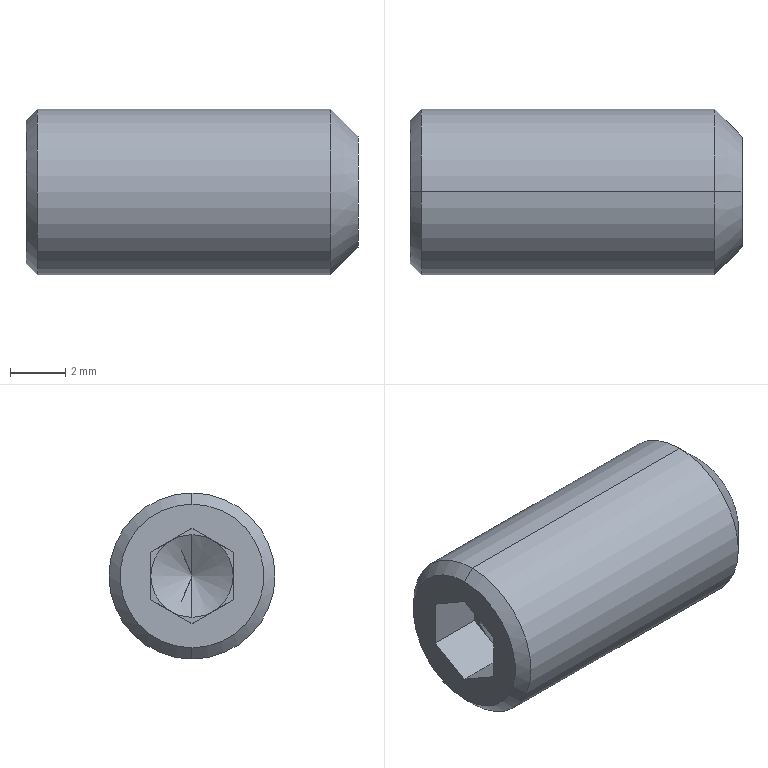Part | SolidWorks | features RevCut 2, Cut 1, LPattern 1, Revolution 1 | 1 solid | 22 faces | box 12 x 6 x 6 mm | volume 312.089 mm3 | plane 14 | cone 6 | cylinder 2 | commonest cylinder face diameters 6 x2
STEP:
#1=CARTESIAN_POINT('',(2.86,0.,0.));
#2=VERTEX_POINT('',#1);
#3=CARTESIAN_POINT('',(2.,0.,1.49));
#4=VERTEX_POINT('',#3);
#5=CARTESIAN_POINT('',(2.86,0.,0.));
#6=DIRECTION('',(-0.5,0.,0.866));
#7=VECTOR('',#6,1000.);
#8=LINE('',#5,#7);
#9=EDGE_CURVE('',#2,#4,#8,.T.);
#10=ORIENTED_EDGE('',*,*,#9,.F.);
#11=CARTESIAN_POINT('',(2.,0.,-1.49));
#12=VERTEX_POINT('',#11);
#13=CARTESIAN_POINT('',(2.86,0.,0.));
#14=DIRECTION('',(-0.5,0.,-0.866));
#15=VECTOR('',#14,1000.);
#16=LINE('',#13,#15);
#17=EDGE_CURVE('',#2,#12,#16,.T.);
#18=ORIENTED_EDGE('',*,*,#17,.T.);
#19=CARTESIAN_POINT('',(2.,-0.7448,-1.29));
#20=VERTEX_POINT('',#19);
#21=CARTESIAN_POINT('',(2.,0.,0.));
#22=DIRECTION('',(-1.,0.,0.));
#23=DIRECTION('',(0.,0.,1.));
#24=AXIS2_PLACEMENT_3D('',#21,#22,#23);
#25=CIRCLE('',#24,1.49);
#26=EDGE_CURVE('',#12,#20,#25,.T.);
#27=ORIENTED_EDGE('',*,*,#26,.T.);
#28=CARTESIAN_POINT('',(2.,-1.49,0.));
#29=VERTEX_POINT('',#28);
#30=CARTESIAN_POINT('',(2.,0.,0.));
#31=DIRECTION('',(-1.,0.,0.));
#32=DIRECTION('',(0.,0.,1.));
#33=AXIS2_PLACEMENT_3D('',#30,#31,#32);
#34=CIRCLE('',#33,1.49);
#35=EDGE_CURVE('',#20,#29,#34,.T.);
#36=ORIENTED_EDGE('',*,*,#35,.T.);
#37=CARTESIAN_POINT('',(2.,-0.7448,1.29));
#38=VERTEX_POINT('',#37);
#39=CARTESIAN_POINT('',(2.,0.,0.));
#40=DIRECTION('',(-1.,0.,0.));
#41=DIRECTION('',(0.,0.,1.));
#42=AXIS2_PLACEMENT_3D('',#39,#40,#41);
#43=CIRCLE('',#42,1.49);
#44=EDGE_CURVE('',#29,#38,#43,.T.);
#45=ORIENTED_EDGE('',*,*,#44,.T.);
#46=CARTESIAN_POINT('',(2.,0.,0.));
#47=DIRECTION('',(-1.,0.,0.));
#48=DIRECTION('',(0.,0.,1.));
#49=AXIS2_PLACEMENT_3D('',#46,#47,#48);
#50=CIRCLE('',#49,1.49);
#51=EDGE_CURVE('',#38,#4,#50,.T.);
#52=ORIENTED_EDGE('',*,*,#51,.T.);
#53=EDGE_LOOP('',(#10,#18,#27,#36,#45,#52));
#54=FACE_OUTER_BOUND('',#53,.T.);
#55=CARTESIAN_POINT('',(-997.14,0.,0.));
#56=DIRECTION('',(-1.,0.,0.));
#57=DIRECTION('',(0.,0.,1.));
#58=AXIS2_PLACEMENT_3D('',#55,#56,#57);
#59=CONICAL_SURFACE('',#58,1732.051,1.047);
#60=ADVANCED_FACE('',(#54),#59,.F.);
#61=CARTESIAN_POINT('',(0.,0.,2.598));
#62=VERTEX_POINT('',#61);
#63=CARTESIAN_POINT('',(0.,0.,-2.598));
#64=VERTEX_POINT('',#63);
#65=CARTESIAN_POINT('',(0.,0.,0.));
#66=DIRECTION('',(-1.,0.,0.));
#67=DIRECTION('',(0.,0.,1.));
#68=AXIS2_PLACEMENT_3D('',#65,#66,#67);
#69=CIRCLE('',#68,2.598);
#70=EDGE_CURVE('',#62,#64,#69,.T.);
#71=ORIENTED_EDGE('',*,*,#70,.F.);
#72=CARTESIAN_POINT('',(0.402,0.,3.));
#73=VERTEX_POINT('',#72);
#74=CARTESIAN_POINT('',(0.402,0.,3.));
#75=DIRECTION('',(0.7071,0.,0.7071));
#76=VECTOR('',#75,1000.);
#77=LINE('',#74,#76);
#78=EDGE_CURVE('',#62,#73,#77,.T.);
#79=ORIENTED_EDGE('',*,*,#78,.T.);
#80=CARTESIAN_POINT('',(0.402,0.,-3.));
#81=VERTEX_POINT('',#80);
#82=CARTESIAN_POINT('',(0.402,0.,0.));
#83=DIRECTION('',(-1.,0.,0.));
#84=DIRECTION('',(0.,0.,1.));
#85=AXIS2_PLACEMENT_3D('',#82,#83,#84);
#86=CIRCLE('',#85,3.);
#87=EDGE_CURVE('',#73,#81,#86,.T.);
#88=ORIENTED_EDGE('',*,*,#87,.T.);
#89=CARTESIAN_POINT('',(0.402,0.,-3.));
#90=DIRECTION('',(0.7071,0.,-0.7071));
#91=VECTOR('',#90,1000.);
#92=LINE('',#89,#91);
#93=EDGE_CURVE('',#64,#81,#92,.T.);
#94=ORIENTED_EDGE('',*,*,#93,.F.);
#95=EDGE_LOOP('',(#71,#79,#88,#94));
#96=FACE_OUTER_BOUND('',#95,.T.);
#97=CARTESIAN_POINT('',(0.402,0.,0.));
#98=DIRECTION('',(1.,0.,0.));
#99=DIRECTION('',(0.,0.,-1.));
#100=AXIS2_PLACEMENT_3D('',#97,#98,#99);
#101=CONICAL_SURFACE('',#100,3.,0.7854);
#102=ADVANCED_FACE('',(#96),#101,.T.);
#103=CARTESIAN_POINT('',(11.,0.,3.));
#104=VERTEX_POINT('',#103);
#105=CARTESIAN_POINT('',(11.,0.,-3.));
#106=VERTEX_POINT('',#105);
#107=CARTESIAN_POINT('',(11.,0.,0.));
#108=DIRECTION('',(-1.,0.,0.));
#109=DIRECTION('',(0.,0.,1.));
#110=AXIS2_PLACEMENT_3D('',#107,#108,#109);
#111=CIRCLE('',#110,3.);
#112=EDGE_CURVE('',#104,#106,#111,.T.);
#113=ORIENTED_EDGE('',*,*,#112,.T.);
#114=CARTESIAN_POINT('',(-0.2778,0.,-3.));
#115=DIRECTION('',(-1.,0.,0.));
#116=VECTOR('',#115,1000.);
#117=LINE('',#114,#116);
#118=EDGE_CURVE('',#106,#81,#117,.T.);
#119=ORIENTED_EDGE('',*,*,#118,.T.);
#120=ORIENTED_EDGE('',*,*,#87,.F.);
#121=CARTESIAN_POINT('',(-0.2778,0.,3.));
#122=DIRECTION('',(-1.,0.,0.));
#123=VECTOR('',#122,1000.);
#124=LINE('',#121,#123);
#125=EDGE_CURVE('',#104,#73,#124,.T.);
#126=ORIENTED_EDGE('',*,*,#125,.F.);
#127=EDGE_LOOP('',(#113,#119,#120,#126));
#128=FACE_OUTER_BOUND('',#127,.T.);
#129=CARTESIAN_POINT('',(-0.2778,0.,0.));
#130=DIRECTION('',(-1.,0.,0.));
#131=DIRECTION('',(0.,0.,1.));
#132=AXIS2_PLACEMENT_3D('',#129,#130,#131);
#133=CYLINDRICAL_SURFACE('',#132,3.);
#134=ADVANCED_FACE('',(#128),#133,.T.);
#135=CARTESIAN_POINT('',(12.,0.,2.));
#136=VERTEX_POINT('',#135);
#137=CARTESIAN_POINT('',(12.,0.,-2.));
#138=VERTEX_POINT('',#137);
#139=CARTESIAN_POINT('',(12.,0.,0.));
#140=DIRECTION('',(-1.,0.,0.));
#141=DIRECTION('',(0.,0.,1.));
#142=AXIS2_PLACEMENT_3D('',#139,#140,#141);
#143=CIRCLE('',#142,2.);
#144=EDGE_CURVE('',#136,#138,#143,.T.);
#145=ORIENTED_EDGE('',*,*,#144,.T.);
#146=CARTESIAN_POINT('',(12.,0.,-2.));
#147=DIRECTION('',(-0.7071,0.,-0.7071));
#148=VECTOR('',#147,1000.);
#149=LINE('',#146,#148);
#150=EDGE_CURVE('',#138,#106,#149,.T.);
#151=ORIENTED_EDGE('',*,*,#150,.T.);
#152=ORIENTED_EDGE('',*,*,#112,.F.);
#153=CARTESIAN_POINT('',(12.,0.,2.));
#154=DIRECTION('',(-0.7071,0.,0.7071));
#155=VECTOR('',#154,1000.);
#156=LINE('',#153,#155);
#157=EDGE_CURVE('',#136,#104,#156,.T.);
#158=ORIENTED_EDGE('',*,*,#157,.F.);
#159=EDGE_LOOP('',(#145,#151,#152,#158));
#160=FACE_OUTER_BOUND('',#159,.T.);
#161=CARTESIAN_POINT('',(12.,0.,0.));
#162=DIRECTION('',(-1.,0.,0.));
#163=DIRECTION('',(0.,0.,1.));
#164=AXIS2_PLACEMENT_3D('',#161,#162,#163);
#165=CONICAL_SURFACE('',#164,2.,0.7854);
#166=ADVANCED_FACE('',(#160),#165,.T.);
#167=CARTESIAN_POINT('',(2.,0.7448,1.29));
#168=VERTEX_POINT('',#167);
#169=CARTESIAN_POINT('',(2.,1.49,0.));
#170=VERTEX_POINT('',#169);
#171=CARTESIAN_POINT('',(2.,0.,0.));
#172=DIRECTION('',(-1.,0.,0.));
#173=DIRECTION('',(0.,0.,1.));
#174=AXIS2_PLACEMENT_3D('',#171,#172,#173);
#175=CIRCLE('',#174,1.49);
#176=EDGE_CURVE('',#168,#170,#175,.T.);
#177=ORIENTED_EDGE('',*,*,#176,.F.);
#178=CARTESIAN_POINT('',(2.,1.49,0.86));
#179=VERTEX_POINT('',#178);
#180=CARTESIAN_POINT('',(2.,0.,1.72));
#181=DIRECTION('',(0.,0.866,-0.5));
#182=VECTOR('',#181,1000.);
#183=LINE('',#180,#182);
#184=EDGE_CURVE('',#168,#179,#183,.T.);
#185=ORIENTED_EDGE('',*,*,#184,.T.);
#186=CARTESIAN_POINT('',(2.,1.49,0.86));
#187=DIRECTION('',(0.,0.,-1.));
#188=VECTOR('',#187,1000.);
#189=LINE('',#186,#188);
#190=EDGE_CURVE('',#179,#170,#189,.T.);
#191=ORIENTED_EDGE('',*,*,#190,.T.);
#192=EDGE_LOOP('',(#177,#185,#191));
#193=FACE_OUTER_BOUND('',#192,.T.);
#194=CARTESIAN_POINT('',(2.,-2.979,0.));
#195=DIRECTION('',(-1.,0.,0.));
#196=DIRECTION('',(0.,0.,1.));
#197=AXIS2_PLACEMENT_3D('',#194,#195,#196);
#198=PLANE('',#197);
#199=ADVANCED_FACE('',(#193),#198,.T.);
#200=CARTESIAN_POINT('',(2.,0.7448,-1.29));
#201=VERTEX_POINT('',#200);
#202=CARTESIAN_POINT('',(2.,0.,0.));
#203=DIRECTION('',(-1.,0.,0.));
#204=DIRECTION('',(0.,0.,1.));
#205=AXIS2_PLACEMENT_3D('',#202,#203,#204);
#206=CIRCLE('',#205,1.49);
#207=EDGE_CURVE('',#170,#201,#206,.T.);
#208=ORIENTED_EDGE('',*,*,#207,.F.);
#209=CARTESIAN_POINT('',(2.,1.49,-0.86));
#210=VERTEX_POINT('',#209);
#211=CARTESIAN_POINT('',(2.,1.49,0.86));
#212=DIRECTION('',(0.,0.,-1.));
#213=VECTOR('',#212,1000.);
#214=LINE('',#211,#213);
#215=EDGE_CURVE('',#170,#210,#214,.T.);
#216=ORIENTED_EDGE('',*,*,#215,.T.);
#217=CARTESIAN_POINT('',(2.,1.49,-0.86));
#218=DIRECTION('',(0.,-0.866,-0.5));
#219=VECTOR('',#218,1000.);
#220=LINE('',#217,#219);
#221=EDGE_CURVE('',#210,#201,#220,.T.);
#222=ORIENTED_EDGE('',*,*,#221,.T.);
#223=EDGE_LOOP('',(#208,#216,#222));
#224=FACE_OUTER_BOUND('',#223,.T.);
#225=CARTESIAN_POINT('',(2.,-2.979,0.));
#226=DIRECTION('',(-1.,0.,0.));
#227=DIRECTION('',(0.,0.,1.));
#228=AXIS2_PLACEMENT_3D('',#225,#226,#227);
#229=PLANE('',#228);
#230=ADVANCED_FACE('',(#224),#229,.T.);
#231=CARTESIAN_POINT('',(2.,0.,0.));
#232=DIRECTION('',(-1.,0.,0.));
#233=DIRECTION('',(0.,0.,1.));
#234=AXIS2_PLACEMENT_3D('',#231,#232,#233);
#235=CIRCLE('',#234,1.49);
#236=EDGE_CURVE('',#201,#12,#235,.T.);
#237=ORIENTED_EDGE('',*,*,#236,.F.);
#238=CARTESIAN_POINT('',(2.,0.,-1.72));
#239=VERTEX_POINT('',#238);
#240=CARTESIAN_POINT('',(2.,1.49,-0.86));
#241=DIRECTION('',(0.,-0.866,-0.5));
#242=VECTOR('',#241,1000.);
#243=LINE('',#240,#242);
#244=EDGE_CURVE('',#201,#239,#243,.T.);
#245=ORIENTED_EDGE('',*,*,#244,.T.);
#246=CARTESIAN_POINT('',(2.,0.,-1.72));
#247=DIRECTION('',(0.,-0.866,0.5));
#248=VECTOR('',#247,1000.);
#249=LINE('',#246,#248);
#250=EDGE_CURVE('',#239,#20,#249,.T.);
#251=ORIENTED_EDGE('',*,*,#250,.T.);
#252=ORIENTED_EDGE('',*,*,#26,.F.);
#253=EDGE_LOOP('',(#237,#245,#251,#252));
#254=FACE_OUTER_BOUND('',#253,.T.);
#255=CARTESIAN_POINT('',(2.,-2.979,0.));
#256=DIRECTION('',(-1.,0.,0.));
#257=DIRECTION('',(0.,0.,1.));
#258=AXIS2_PLACEMENT_3D('',#255,#256,#257);
#259=PLANE('',#258);
#260=ADVANCED_FACE('',(#254),#259,.T.);
#261=ORIENTED_EDGE('',*,*,#35,.F.);
#262=CARTESIAN_POINT('',(2.,-1.49,-0.86));
#263=VERTEX_POINT('',#262);
#264=CARTESIAN_POINT('',(2.,0.,-1.72));
#265=DIRECTION('',(0.,-0.866,0.5));
#266=VECTOR('',#265,1000.);
#267=LINE('',#264,#266);
#268=EDGE_CURVE('',#20,#263,#267,.T.);
#269=ORIENTED_EDGE('',*,*,#268,.T.);
#270=CARTESIAN_POINT('',(2.,-1.49,-0.86));
#271=DIRECTION('',(0.,0.,1.));
#272=VECTOR('',#271,1000.);
#273=LINE('',#270,#272);
#274=EDGE_CURVE('',#263,#29,#273,.T.);
#275=ORIENTED_EDGE('',*,*,#274,.T.);
#276=EDGE_LOOP('',(#261,#269,#275));
#277=FACE_OUTER_BOUND('',#276,.T.);
#278=CARTESIAN_POINT('',(2.,-2.979,0.));
#279=DIRECTION('',(-1.,0.,0.));
#280=DIRECTION('',(0.,0.,1.));
#281=AXIS2_PLACEMENT_3D('',#278,#279,#280);
#282=PLANE('',#281);
#283=ADVANCED_FACE('',(#277),#282,.T.);
#284=ORIENTED_EDGE('',*,*,#44,.F.);
#285=CARTESIAN_POINT('',(2.,-1.49,0.86));
#286=VERTEX_POINT('',#285);
#287=CARTESIAN_POINT('',(2.,-1.49,-0.86));
#288=DIRECTION('',(0.,0.,1.));
#289=VECTOR('',#288,1000.);
#290=LINE('',#287,#289);
#291=EDGE_CURVE('',#29,#286,#290,.T.);
#292=ORIENTED_EDGE('',*,*,#291,.T.);
#293=CARTESIAN_POINT('',(2.,-1.49,0.86));
#294=DIRECTION('',(0.,0.866,0.5));
#295=VECTOR('',#294,1000.);
#296=LINE('',#293,#295);
#297=EDGE_CURVE('',#286,#38,#296,.T.);
#298=ORIENTED_EDGE('',*,*,#297,.T.);
#299=EDGE_LOOP('',(#284,#292,#298));
#300=FACE_OUTER_BOUND('',#299,.T.);
#301=CARTESIAN_POINT('',(2.,-2.979,0.));
#302=DIRECTION('',(-1.,0.,0.));
#303=DIRECTION('',(0.,0.,1.));
#304=AXIS2_PLACEMENT_3D('',#301,#302,#303);
#305=PLANE('',#304);
#306=ADVANCED_FACE('',(#300),#305,.T.);
#307=CARTESIAN_POINT('',(0.,-1.49,-0.86));
#308=VERTEX_POINT('',#307);
#309=CARTESIAN_POINT('',(0.,-1.49,0.86));
#310=VERTEX_POINT('',#309);
#311=CARTESIAN_POINT('',(0.,-1.49,-0.86));
#312=DIRECTION('',(0.,0.,1.));
#313=VECTOR('',#312,1000.);
#314=LINE('',#311,#313);
#315=EDGE_CURVE('',#308,#310,#314,.T.);
#316=ORIENTED_EDGE('',*,*,#315,.F.);
#317=CARTESIAN_POINT('',(0.,0.,-1.72));
#318=VERTEX_POINT('',#317);
#319=CARTESIAN_POINT('',(0.,0.,-1.72));
#320=DIRECTION('',(0.,-0.866,0.5));
#321=VECTOR('',#320,1000.);
#322=LINE('',#319,#321);
#323=EDGE_CURVE('',#318,#308,#322,.T.);
#324=ORIENTED_EDGE('',*,*,#323,.F.);
#325=CARTESIAN_POINT('',(0.,1.49,-0.86));
#326=VERTEX_POINT('',#325);
#327=CARTESIAN_POINT('',(0.,1.49,-0.86));
#328=DIRECTION('',(0.,-0.866,-0.5));
#329=VECTOR('',#328,1000.);
#330=LINE('',#327,#329);
#331=EDGE_CURVE('',#326,#318,#330,.T.);
#332=ORIENTED_EDGE('',*,*,#331,.F.);
#333=CARTESIAN_POINT('',(0.,1.49,0.86));
#334=VERTEX_POINT('',#333);
#335=CARTESIAN_POINT('',(0.,1.49,0.86));
#336=DIRECTION('',(0.,0.,-1.));
#337=VECTOR('',#336,1000.);
#338=LINE('',#335,#337);
#339=EDGE_CURVE('',#334,#326,#338,.T.);
#340=ORIENTED_EDGE('',*,*,#339,.F.);
#341=CARTESIAN_POINT('',(0.,0.,1.72));
#342=VERTEX_POINT('',#341);
#343=CARTESIAN_POINT('',(0.,0.,1.72));
#344=DIRECTION('',(0.,0.866,-0.5));
#345=VECTOR('',#344,1000.);
#346=LINE('',#343,#345);
#347=EDGE_CURVE('',#342,#334,#346,.T.);
#348=ORIENTED_EDGE('',*,*,#347,.F.);
#349=CARTESIAN_POINT('',(0.,-1.49,0.86));
#350=DIRECTION('',(0.,0.866,0.5));
#351=VECTOR('',#350,1000.);
#352=LINE('',#349,#351);
#353=EDGE_CURVE('',#310,#342,#352,.T.);
#354=ORIENTED_EDGE('',*,*,#353,.F.);
#355=EDGE_LOOP('',(#316,#324,#332,#340,#348,#354));
#356=FACE_BOUND('',#355,.T.);
#357=CARTESIAN_POINT('',(0.,0.,0.));
#358=DIRECTION('',(-1.,0.,0.));
#359=DIRECTION('',(0.,0.,1.));
#360=AXIS2_PLACEMENT_3D('',#357,#358,#359);
#361=CIRCLE('',#360,2.598);
#362=EDGE_CURVE('',#64,#62,#361,.T.);
#363=ORIENTED_EDGE('',*,*,#362,.T.);
#364=ORIENTED_EDGE('',*,*,#70,.T.);
#365=EDGE_LOOP('',(#363,#364));
#366=FACE_OUTER_BOUND('',#365,.T.);
#367=CARTESIAN_POINT('',(0.,2.598,0.));
#368=DIRECTION('',(1.,0.,0.));
#369=DIRECTION('',(0.,0.,-1.));
#370=AXIS2_PLACEMENT_3D('',#367,#368,#369);
#371=PLANE('',#370);
#372=ADVANCED_FACE('',(#356,#366),#371,.F.);
#373=ORIENTED_EDGE('',*,*,#144,.F.);
#374=CARTESIAN_POINT('',(12.,0.,0.));
#375=DIRECTION('',(-1.,0.,0.));
#376=DIRECTION('',(0.,0.,1.));
#377=AXIS2_PLACEMENT_3D('',#374,#375,#376);
#378=CIRCLE('',#377,2.);
#379=EDGE_CURVE('',#138,#136,#378,.T.);
#380=ORIENTED_EDGE('',*,*,#379,.F.);
#381=EDGE_LOOP('',(#373,#380));
#382=FACE_OUTER_BOUND('',#381,.T.);
#383=CARTESIAN_POINT('',(12.,0.,0.));
#384=DIRECTION('',(-1.,0.,0.));
#385=DIRECTION('',(0.,0.,1.));
#386=AXIS2_PLACEMENT_3D('',#383,#384,#385);
#387=PLANE('',#386);
#388=ADVANCED_FACE('',(#382),#387,.F.);
#389=ORIENTED_EDGE('',*,*,#150,.F.);
#390=ORIENTED_EDGE('',*,*,#379,.T.);
#391=ORIENTED_EDGE('',*,*,#157,.T.);
#392=CARTESIAN_POINT('',(11.,0.,0.));
#393=DIRECTION('',(-1.,0.,0.));
#394=DIRECTION('',(0.,0.,1.));
#395=AXIS2_PLACEMENT_3D('',#392,#393,#394);
#396=CIRCLE('',#395,3.);
#397=EDGE_CURVE('',#106,#104,#396,.T.);
#398=ORIENTED_EDGE('',*,*,#397,.F.);
#399=EDGE_LOOP('',(#389,#390,#391,#398));
#400=FACE_OUTER_BOUND('',#399,.T.);
#401=CARTESIAN_POINT('',(12.,0.,0.));
#402=DIRECTION('',(-1.,0.,0.));
#403=DIRECTION('',(0.,0.,1.));
#404=AXIS2_PLACEMENT_3D('',#401,#402,#403);
#405=CONICAL_SURFACE('',#404,2.,0.7854);
#406=ADVANCED_FACE('',(#400),#405,.T.);
#407=ORIENTED_EDGE('',*,*,#118,.F.);
#408=ORIENTED_EDGE('',*,*,#397,.T.);
#409=ORIENTED_EDGE('',*,*,#125,.T.);
#410=CARTESIAN_POINT('',(0.402,0.,0.));
#411=DIRECTION('',(-1.,0.,0.));
#412=DIRECTION('',(0.,0.,1.));
#413=AXIS2_PLACEMENT_3D('',#410,#411,#412);
#414=CIRCLE('',#413,3.);
#415=EDGE_CURVE('',#81,#73,#414,.T.);
#416=ORIENTED_EDGE('',*,*,#415,.F.);
#417=EDGE_LOOP('',(#407,#408,#409,#416));
#418=FACE_OUTER_BOUND('',#417,.T.);
#419=CARTESIAN_POINT('',(-0.2778,0.,0.));
#420=DIRECTION('',(-1.,0.,0.));
#421=DIRECTION('',(0.,0.,1.));
#422=AXIS2_PLACEMENT_3D('',#419,#420,#421);
#423=CYLINDRICAL_SURFACE('',#422,3.);
#424=ADVANCED_FACE('',(#418),#423,.T.);
#425=ORIENTED_EDGE('',*,*,#78,.F.);
#426=ORIENTED_EDGE('',*,*,#362,.F.);
#427=ORIENTED_EDGE('',*,*,#93,.T.);
#428=ORIENTED_EDGE('',*,*,#415,.T.);
#429=EDGE_LOOP('',(#425,#426,#427,#428));
#430=FACE_OUTER_BOUND('',#429,.T.);
#431=CARTESIAN_POINT('',(0.402,0.,0.));
#432=DIRECTION('',(1.,0.,0.));
#433=DIRECTION('',(0.,0.,-1.));
#434=AXIS2_PLACEMENT_3D('',#431,#432,#433);
#435=CONICAL_SURFACE('',#434,3.,0.7854);
#436=ADVANCED_FACE('',(#430),#435,.T.);
#437=ORIENTED_EDGE('',*,*,#323,.T.);
#438=CARTESIAN_POINT('',(2.,-1.49,-0.86));
#439=DIRECTION('',(-1.,0.,0.));
#440=VECTOR('',#439,1000.);
#441=LINE('',#438,#440);
#442=EDGE_CURVE('',#263,#308,#441,.T.);
#443=ORIENTED_EDGE('',*,*,#442,.F.);
#444=ORIENTED_EDGE('',*,*,#268,.F.);
#445=ORIENTED_EDGE('',*,*,#250,.F.);
#446=CARTESIAN_POINT('',(2.,0.,-1.72));
#447=DIRECTION('',(-1.,0.,0.));
#448=VECTOR('',#447,1000.);
#449=LINE('',#446,#448);
#450=EDGE_CURVE('',#239,#318,#449,.T.);
#451=ORIENTED_EDGE('',*,*,#450,.T.);
#452=EDGE_LOOP('',(#437,#443,#444,#445,#451));
#453=FACE_OUTER_BOUND('',#452,.T.);
#454=CARTESIAN_POINT('',(2.,0.,-1.72));
#455=DIRECTION('',(0.,-0.5,-0.866));
#456=DIRECTION('',(0.,0.866,-0.5));
#457=AXIS2_PLACEMENT_3D('',#454,#455,#456);
#458=PLANE('',#457);
#459=ADVANCED_FACE('',(#453),#458,.F.);
#460=ORIENTED_EDGE('',*,*,#331,.T.);
#461=ORIENTED_EDGE('',*,*,#450,.F.);
#462=ORIENTED_EDGE('',*,*,#244,.F.);
#463=ORIENTED_EDGE('',*,*,#221,.F.);
#464=CARTESIAN_POINT('',(2.,1.49,-0.86));
#465=DIRECTION('',(-1.,0.,0.));
#466=VECTOR('',#465,1000.);
#467=LINE('',#464,#466);
#468=EDGE_CURVE('',#210,#326,#467,.T.);
#469=ORIENTED_EDGE('',*,*,#468,.T.);
#470=EDGE_LOOP('',(#460,#461,#462,#463,#469));
#471=FACE_OUTER_BOUND('',#470,.T.);
#472=CARTESIAN_POINT('',(2.,1.49,-0.86));
#473=DIRECTION('',(0.,0.5,-0.866));
#474=DIRECTION('',(0.,0.866,0.5));
#475=AXIS2_PLACEMENT_3D('',#472,#473,#474);
#476=PLANE('',#475);
#477=ADVANCED_FACE('',(#471),#476,.F.);
#478=ORIENTED_EDGE('',*,*,#339,.T.);
#479=ORIENTED_EDGE('',*,*,#468,.F.);
#480=ORIENTED_EDGE('',*,*,#215,.F.);
#481=ORIENTED_EDGE('',*,*,#190,.F.);
#482=CARTESIAN_POINT('',(2.,1.49,0.86));
#483=DIRECTION('',(-1.,0.,0.));
#484=VECTOR('',#483,1000.);
#485=LINE('',#482,#484);
#486=EDGE_CURVE('',#179,#334,#485,.T.);
#487=ORIENTED_EDGE('',*,*,#486,.T.);
#488=EDGE_LOOP('',(#478,#479,#480,#481,#487));
#489=FACE_OUTER_BOUND('',#488,.T.);
#490=CARTESIAN_POINT('',(2.,1.49,0.86));
#491=DIRECTION('',(0.,1.,0.));
#492=DIRECTION('',(0.,0.,1.));
#493=AXIS2_PLACEMENT_3D('',#490,#491,#492);
#494=PLANE('',#493);
#495=ADVANCED_FACE('',(#489),#494,.F.);
#496=ORIENTED_EDGE('',*,*,#347,.T.);
#497=ORIENTED_EDGE('',*,*,#486,.F.);
#498=ORIENTED_EDGE('',*,*,#184,.F.);
#499=CARTESIAN_POINT('',(2.,0.,1.72));
#500=VERTEX_POINT('',#499);
#501=CARTESIAN_POINT('',(2.,0.,1.72));
#502=DIRECTION('',(0.,0.866,-0.5));
#503=VECTOR('',#502,1000.);
#504=LINE('',#501,#503);
#505=EDGE_CURVE('',#500,#168,#504,.T.);
#506=ORIENTED_EDGE('',*,*,#505,.F.);
#507=CARTESIAN_POINT('',(2.,0.,1.72));
#508=DIRECTION('',(-1.,0.,0.));
#509=VECTOR('',#508,1000.);
#510=LINE('',#507,#509);
#511=EDGE_CURVE('',#500,#342,#510,.T.);
#512=ORIENTED_EDGE('',*,*,#511,.T.);
#513=EDGE_LOOP('',(#496,#497,#498,#506,#512));
#514=FACE_OUTER_BOUND('',#513,.T.);
#515=CARTESIAN_POINT('',(2.,0.,1.72));
#516=DIRECTION('',(0.,0.5,0.866));
#517=DIRECTION('',(0.,-0.866,0.5));
#518=AXIS2_PLACEMENT_3D('',#515,#516,#517);
#519=PLANE('',#518);
#520=ADVANCED_FACE('',(#514),#519,.F.);
#521=ORIENTED_EDGE('',*,*,#353,.T.);
#522=ORIENTED_EDGE('',*,*,#511,.F.);
#523=CARTESIAN_POINT('',(2.,-1.49,0.86));
#524=DIRECTION('',(0.,0.866,0.5));
#525=VECTOR('',#524,1000.);
#526=LINE('',#523,#525);
#527=EDGE_CURVE('',#38,#500,#526,.T.);
#528=ORIENTED_EDGE('',*,*,#527,.F.);
#529=ORIENTED_EDGE('',*,*,#297,.F.);
#530=CARTESIAN_POINT('',(2.,-1.49,0.86));
#531=DIRECTION('',(-1.,0.,0.));
#532=VECTOR('',#531,1000.);
#533=LINE('',#530,#532);
#534=EDGE_CURVE('',#286,#310,#533,.T.);
#535=ORIENTED_EDGE('',*,*,#534,.T.);
#536=EDGE_LOOP('',(#521,#522,#528,#529,#535));
#537=FACE_OUTER_BOUND('',#536,.T.);
#538=CARTESIAN_POINT('',(2.,-1.49,0.86));
#539=DIRECTION('',(0.,-0.5,0.866));
#540=DIRECTION('',(0.,-0.866,-0.5));
#541=AXIS2_PLACEMENT_3D('',#538,#539,#540);
#542=PLANE('',#541);
#543=ADVANCED_FACE('',(#537),#542,.F.);
#544=ORIENTED_EDGE('',*,*,#315,.T.);
#545=ORIENTED_EDGE('',*,*,#534,.F.);
#546=ORIENTED_EDGE('',*,*,#291,.F.);
#547=ORIENTED_EDGE('',*,*,#274,.F.);
#548=ORIENTED_EDGE('',*,*,#442,.T.);
#549=EDGE_LOOP('',(#544,#545,#546,#547,#548));
#550=FACE_OUTER_BOUND('',#549,.T.);
#551=CARTESIAN_POINT('',(2.,-1.49,-0.86));
#552=DIRECTION('',(0.,-1.,0.));
#553=DIRECTION('',(0.,0.,-1.));
#554=AXIS2_PLACEMENT_3D('',#551,#552,#553);
#555=PLANE('',#554);
#556=ADVANCED_FACE('',(#550),#555,.F.);
#557=ORIENTED_EDGE('',*,*,#51,.F.);
#558=ORIENTED_EDGE('',*,*,#527,.T.);
#559=ORIENTED_EDGE('',*,*,#505,.T.);
#560=CARTESIAN_POINT('',(2.,0.,0.));
#561=DIRECTION('',(-1.,0.,0.));
#562=DIRECTION('',(0.,0.,1.));
#563=AXIS2_PLACEMENT_3D('',#560,#561,#562);
#564=CIRCLE('',#563,1.49);
#565=EDGE_CURVE('',#4,#168,#564,.T.);
#566=ORIENTED_EDGE('',*,*,#565,.F.);
#567=EDGE_LOOP('',(#557,#558,#559,#566));
#568=FACE_OUTER_BOUND('',#567,.T.);
#569=CARTESIAN_POINT('',(2.,-2.979,0.));
#570=DIRECTION('',(-1.,0.,0.));
#571=DIRECTION('',(0.,0.,1.));
#572=AXIS2_PLACEMENT_3D('',#569,#570,#571);
#573=PLANE('',#572);
#574=ADVANCED_FACE('',(#568),#573,.T.);
#575=ORIENTED_EDGE('',*,*,#17,.F.);
#576=ORIENTED_EDGE('',*,*,#9,.T.);
#577=ORIENTED_EDGE('',*,*,#565,.T.);
#578=ORIENTED_EDGE('',*,*,#176,.T.);
#579=ORIENTED_EDGE('',*,*,#207,.T.);
#580=ORIENTED_EDGE('',*,*,#236,.T.);
#581=EDGE_LOOP('',(#575,#576,#577,#578,#579,#580));
#582=FACE_OUTER_BOUND('',#581,.T.);
#583=CARTESIAN_POINT('',(-997.14,0.,0.));
#584=DIRECTION('',(-1.,0.,0.));
#585=DIRECTION('',(0.,0.,1.));
#586=AXIS2_PLACEMENT_3D('',#583,#584,#585);
#587=CONICAL_SURFACE('',#586,1732.051,1.047);
#588=ADVANCED_FACE('',(#582),#587,.F.);
#589=CLOSED_SHELL('',(#60,#102,#134,#166,#199,#230,#260,#283,#306,#372,#388,#406,#424,#436,#459,#477,#495,#520,#543,#556,#574,#588));
#590=MANIFOLD_SOLID_BREP('',#589);
#591=CARTESIAN_POINT('',(0.,0.,0.));
#592=DIRECTION('',(0.,0.,1.));
#593=DIRECTION('',(1.,0.,0.));
#594=AXIS2_PLACEMENT_3D('',#591,#592,#593);
#595=(LENGTH_UNIT()NAMED_UNIT(*)SI_UNIT(.MILLI.,.METRE.));
#596=UNCERTAINTY_MEASURE_WITH_UNIT(LENGTH_MEASURE(0.00001),#595,'','');
#597=(NAMED_UNIT(*)PLANE_ANGLE_UNIT()SI_UNIT($,.RADIAN.));
#598=(NAMED_UNIT(*)SI_UNIT($,.STERADIAN.)SOLID_ANGLE_UNIT());
#599=(GEOMETRIC_REPRESENTATION_CONTEXT(3)GLOBAL_UNCERTAINTY_ASSIGNED_CONTEXT((#596))GLOBAL_UNIT_ASSIGNED_CONTEXT((#595,#597,#598))REPRESENTATION_CONTEXT('',''));
#600=ADVANCED_BREP_SHAPE_REPRESENTATION('',(#590,#594),#599);